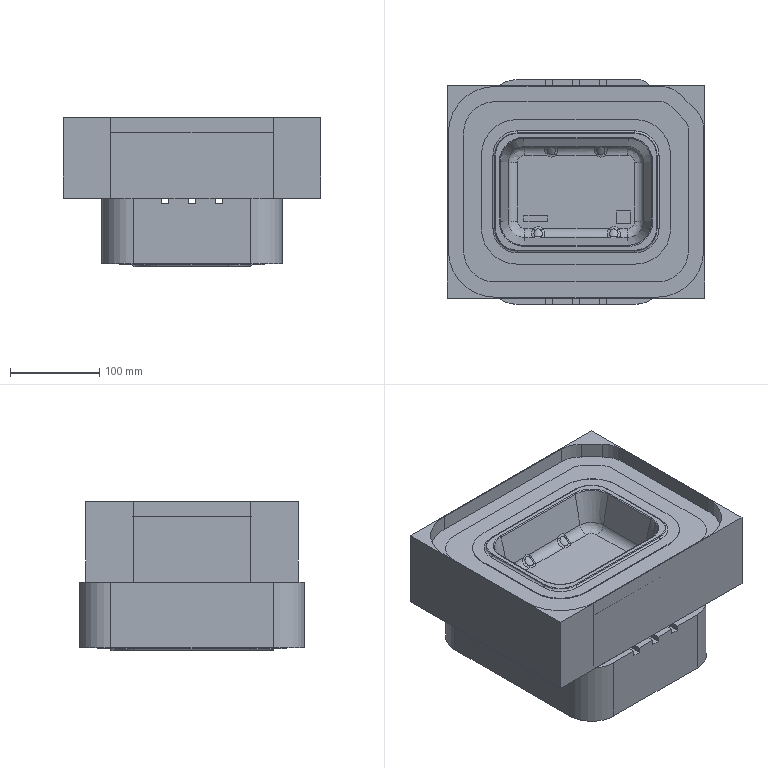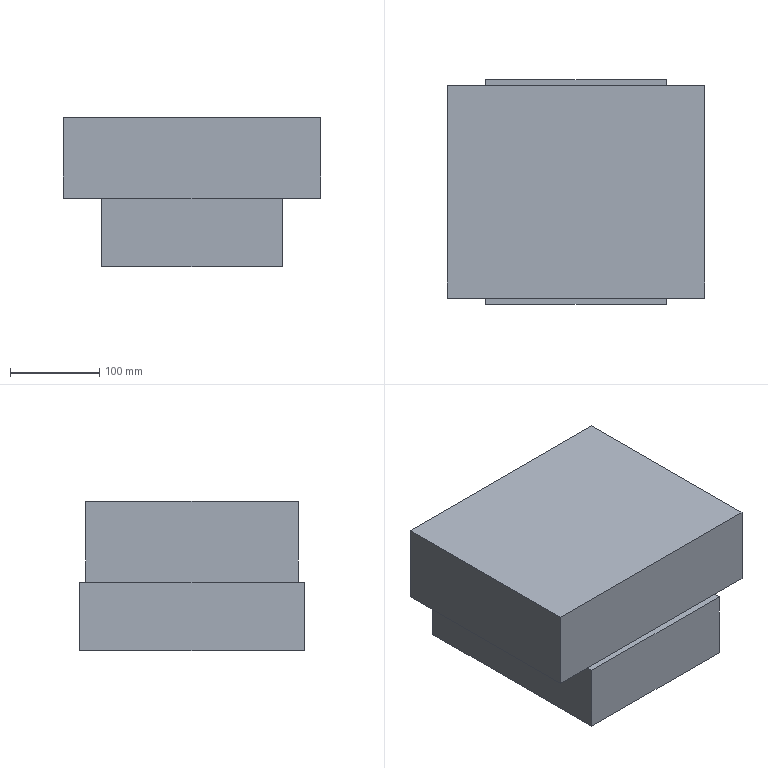CAM job | NX | 3-axis milling, drilling | part box 287.436 x 251.436 x 167.016 mm | stock box 287.436 x 251.436 x 167.016 mm
Tools:
number,name,description,diameter,corner_radius,flute_length,length,flutes
0,V2.0,Drilling Tool,2.0,0.0,35.0,50.0,2
0,V8.0,Drilling Tool,8.0,0.0,35.0,50.0,2
0,D12,No Description,12.0,0.0,50.0,70.0,2
0,D8,No Description,8.0,0.0,0.0,40.0,2
0,D16R0.8,No Description,16.0,0.8,50.0,90.0,2
0,R2,No Description,4.0,2.0,0.0,20.0,2
Operations:
program,operation,operation_type,tool,method,geometry_group,spindle_rpm,surface_speed,feed_per_tooth,feed_cut,feed_plunge,cut_length_mm,path_length_mm,cut_time_min,machine_time_min
B-1,01,CavityMilling,D16R0.8,METHOD,23C,7000.0,1099.0,0.3214,4500.0,100.0,406781.184,416913.517,90.396,91.409
B-2,02,CavityMilling,D8,METHOD,23C,7000.0,1099.0,0.3214,4500.0,100.0,14667.801,19189.545,3.26,3.712
B-3,05,FaceMilling,D12,METHOD,23C,7000.0,1099.0,0.2857,4000.0,100.0,4869.777,5201.413,1.217,1.251
B-4,06,SurfaceContour,R2,METHOD,23C,8000.0,251.0,0.2812,4500.0,100.0,176296.356,176667.174,39.177,39.214
B-4,04,Engraving,R2,METHOD,23C,9000.0,113.0,0.1111,2000.0,100.0,2088.813,15466.611,1.942,3.28
B-5,DRILLING,Operation,V2.0,METHOD,23C,2000.0,75.0,0.0375,150.0,0.0,195.0,1948.107,1.3,1.475
B-6,07,PlanarMilling,D16R0.8,METHOD,23C,7000.0,571.0,0.2857,4000.0,100.0,85673.216,86078.834,21.418,21.459
C-1,CAVITY_MILL_2,CavityMilling,D8,METHOD,24D,7000.0,1099.0,0.3214,4500.0,100.0,70963.306,85475.847,15.77,17.221
C-2,DRILLING_1,Operation,V2.0,METHOD,24D,2000.0,75.0,0.0375,150.0,0.0,195.0,3115.482,1.3,1.592
C-3,DRILLING_1_COPY,Operation,V8.0,METHOD,24D,2000.0,75.0,0.0375,150.0,0.0,1248.0,3467.544,8.32,8.542
C-3,DRILLING_1_COPY_COPY,Operation,V8.0,METHOD,24D,2000.0,75.0,0.0375,150.0,0.0,105.0,986.095,0.7,0.7881